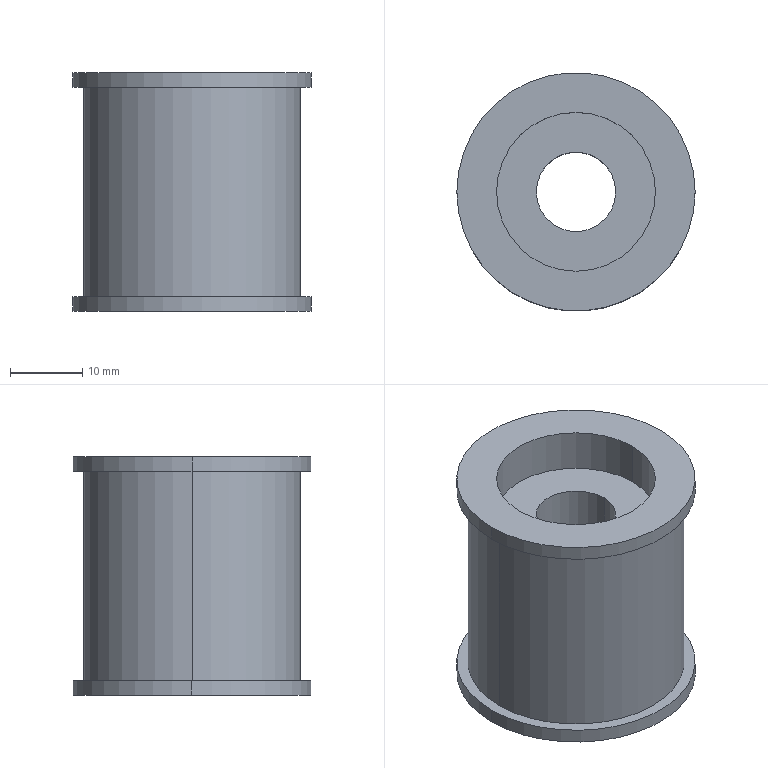Part | STEP file | (PA01.001.LX016) Idler B | 1 solid | 18 faces | box 33 x 33 x 33 mm | volume 17363 mm3 | cylinder 12 | plane 6 | commonest cylinder face diameters 22 x4 33 x4 11 x2 30 x2
STEP:
#1=CARTESIAN_POINT('',(0.,0.,0.));
#2=DIRECTION('',(0.,0.,1.));
#3=DIRECTION('',(1.,0.,0.));
#4=AXIS2_PLACEMENT_3D('',#1,#2,#3);
#5=CARTESIAN_POINT('',(-11.,0.,-10.5));
#6=VERTEX_POINT('',#5);
#7=CARTESIAN_POINT('',(-11.,0.,-16.5));
#8=VERTEX_POINT('',#7);
#9=CARTESIAN_POINT('',(-11.,0.,-10.5));
#10=DIRECTION('',(0.,0.,-1.));
#11=VECTOR('',#10,1.);
#12=LINE('',#9,#11);
#13=CARTESIAN_POINT('',(0.,0.,-10.5));
#14=DIRECTION('',(0.,0.,-1.));
#15=DIRECTION('',(-1.,0.,0.));
#16=AXIS2_PLACEMENT_3D('',#13,#14,#15);
#17=CYLINDRICAL_SURFACE('',#16,11.);
#18=CARTESIAN_POINT('',(6.283,0.));
#19=DIRECTION('',(0.,1.));
#20=VECTOR('',#19,1.);
#21=LINE('',#18,#20);
#22=(GEOMETRIC_REPRESENTATION_CONTEXT(2)PARAMETRIC_REPRESENTATION_CONTEXT()REPRESENTATION_CONTEXT('',''));
#23=DEFINITIONAL_REPRESENTATION('',(#21),#22);
#24=PCURVE('',#17,#23);
#25=CARTESIAN_POINT('',(0.,0.,-10.5));
#26=DIRECTION('',(0.,0.,-1.));
#27=DIRECTION('',(-1.,0.,0.));
#28=AXIS2_PLACEMENT_3D('',#25,#26,#27);
#29=CYLINDRICAL_SURFACE('',#28,11.);
#30=CARTESIAN_POINT('',(0.,0.));
#31=DIRECTION('',(0.,1.));
#32=VECTOR('',#31,1.);
#33=LINE('',#30,#32);
#34=(GEOMETRIC_REPRESENTATION_CONTEXT(2)PARAMETRIC_REPRESENTATION_CONTEXT()REPRESENTATION_CONTEXT('',''));
#35=DEFINITIONAL_REPRESENTATION('',(#33),#34);
#36=PCURVE('',#29,#35);
#37=SURFACE_CURVE('',#12,(#24,#36),.PCURVE_S1.);
#38=EDGE_CURVE('',#6,#8,#37,.T.);
#39=ORIENTED_EDGE('',*,*,#38,.T.);
#40=CARTESIAN_POINT('',(11.,0.,-16.5));
#41=VERTEX_POINT('',#40);
#42=CARTESIAN_POINT('',(0.,0.,-16.5));
#43=DIRECTION('',(0.,0.,-1.));
#44=DIRECTION('',(-1.,0.,0.));
#45=AXIS2_PLACEMENT_3D('',#42,#43,#44);
#46=CIRCLE('',#45,11.);
#47=CARTESIAN_POINT('',(0.,6.));
#48=DIRECTION('',(1.,0.));
#49=VECTOR('',#48,1.);
#50=LINE('',#47,#49);
#51=(GEOMETRIC_REPRESENTATION_CONTEXT(2)PARAMETRIC_REPRESENTATION_CONTEXT()REPRESENTATION_CONTEXT('',''));
#52=DEFINITIONAL_REPRESENTATION('',(#50),#51);
#53=PCURVE('',#17,#52);
#54=CARTESIAN_POINT('',(0.,0.,-16.5));
#55=DIRECTION('',(0.,0.,-1.));
#56=DIRECTION('',(-1.,0.,0.));
#57=AXIS2_PLACEMENT_3D('',#54,#55,#56);
#58=PLANE('',#57);
#59=CARTESIAN_POINT('',(0.,0.));
#60=DIRECTION('',(1.,0.));
#61=AXIS2_PLACEMENT_2D('',#59,#60);
#62=CIRCLE('',#61,11.);
#63=(GEOMETRIC_REPRESENTATION_CONTEXT(2)PARAMETRIC_REPRESENTATION_CONTEXT()REPRESENTATION_CONTEXT('',''));
#64=DEFINITIONAL_REPRESENTATION('',(#62),#63);
#65=PCURVE('',#58,#64);
#66=SURFACE_CURVE('',#46,(#53,#65),.PCURVE_S1.);
#67=EDGE_CURVE('',#41,#8,#66,.T.);
#68=ORIENTED_EDGE('',*,*,#67,.F.);
#69=CARTESIAN_POINT('',(11.,0.,-10.5));
#70=VERTEX_POINT('',#69);
#71=CARTESIAN_POINT('',(11.,0.,-10.5));
#72=DIRECTION('',(0.,0.,-1.));
#73=VECTOR('',#72,1.);
#74=LINE('',#71,#73);
#75=CARTESIAN_POINT('',(3.142,0.));
#76=DIRECTION('',(0.,1.));
#77=VECTOR('',#76,1.);
#78=LINE('',#75,#77);
#79=(GEOMETRIC_REPRESENTATION_CONTEXT(2)PARAMETRIC_REPRESENTATION_CONTEXT()REPRESENTATION_CONTEXT('',''));
#80=DEFINITIONAL_REPRESENTATION('',(#78),#79);
#81=PCURVE('',#17,#80);
#82=CARTESIAN_POINT('',(3.142,0.));
#83=DIRECTION('',(0.,1.));
#84=VECTOR('',#83,1.);
#85=LINE('',#82,#84);
#86=(GEOMETRIC_REPRESENTATION_CONTEXT(2)PARAMETRIC_REPRESENTATION_CONTEXT()REPRESENTATION_CONTEXT('',''));
#87=DEFINITIONAL_REPRESENTATION('',(#85),#86);
#88=PCURVE('',#29,#87);
#89=SURFACE_CURVE('',#74,(#81,#88),.PCURVE_S1.);
#90=EDGE_CURVE('',#70,#41,#89,.T.);
#91=ORIENTED_EDGE('',*,*,#90,.F.);
#92=CARTESIAN_POINT('',(0.,0.,-10.5));
#93=DIRECTION('',(0.,0.,-1.));
#94=DIRECTION('',(-1.,0.,0.));
#95=AXIS2_PLACEMENT_3D('',#92,#93,#94);
#96=CIRCLE('',#95,11.);
#97=CARTESIAN_POINT('',(0.,0.));
#98=DIRECTION('',(1.,0.));
#99=VECTOR('',#98,1.);
#100=LINE('',#97,#99);
#101=(GEOMETRIC_REPRESENTATION_CONTEXT(2)PARAMETRIC_REPRESENTATION_CONTEXT()REPRESENTATION_CONTEXT('',''));
#102=DEFINITIONAL_REPRESENTATION('',(#100),#101);
#103=PCURVE('',#17,#102);
#104=CARTESIAN_POINT('',(0.,0.,-10.5));
#105=DIRECTION('',(0.,0.,-1.));
#106=DIRECTION('',(-1.,0.,0.));
#107=AXIS2_PLACEMENT_3D('',#104,#105,#106);
#108=PLANE('',#107);
#109=CARTESIAN_POINT('',(0.,0.));
#110=DIRECTION('',(1.,0.));
#111=AXIS2_PLACEMENT_2D('',#109,#110);
#112=CIRCLE('',#111,11.);
#113=(GEOMETRIC_REPRESENTATION_CONTEXT(2)PARAMETRIC_REPRESENTATION_CONTEXT()REPRESENTATION_CONTEXT('',''));
#114=DEFINITIONAL_REPRESENTATION('',(#112),#113);
#115=PCURVE('',#108,#114);
#116=SURFACE_CURVE('',#96,(#103,#115),.PCURVE_S1.);
#117=EDGE_CURVE('',#70,#6,#116,.T.);
#118=ORIENTED_EDGE('',*,*,#117,.T.);
#119=EDGE_LOOP('',(#39,#68,#91,#118));
#120=FACE_BOUND('',#119,.F.);
#121=ADVANCED_FACE('',(#120),#17,.F.);
#122=CARTESIAN_POINT('',(11.,0.,10.5));
#123=VERTEX_POINT('',#122);
#124=CARTESIAN_POINT('',(11.,0.,16.5));
#125=VERTEX_POINT('',#124);
#126=CARTESIAN_POINT('',(11.,0.,10.5));
#127=DIRECTION('',(0.,0.,1.));
#128=VECTOR('',#127,1.);
#129=LINE('',#126,#128);
#130=CARTESIAN_POINT('',(0.,0.,10.5));
#131=DIRECTION('',(0.,0.,1.));
#132=DIRECTION('',(1.,0.,0.));
#133=AXIS2_PLACEMENT_3D('',#130,#131,#132);
#134=CYLINDRICAL_SURFACE('',#133,11.);
#135=CARTESIAN_POINT('',(6.283,0.));
#136=DIRECTION('',(0.,1.));
#137=VECTOR('',#136,1.);
#138=LINE('',#135,#137);
#139=(GEOMETRIC_REPRESENTATION_CONTEXT(2)PARAMETRIC_REPRESENTATION_CONTEXT()REPRESENTATION_CONTEXT('',''));
#140=DEFINITIONAL_REPRESENTATION('',(#138),#139);
#141=PCURVE('',#134,#140);
#142=CARTESIAN_POINT('',(0.,0.,10.5));
#143=DIRECTION('',(0.,0.,1.));
#144=DIRECTION('',(1.,0.,0.));
#145=AXIS2_PLACEMENT_3D('',#142,#143,#144);
#146=CYLINDRICAL_SURFACE('',#145,11.);
#147=CARTESIAN_POINT('',(0.,0.));
#148=DIRECTION('',(0.,1.));
#149=VECTOR('',#148,1.);
#150=LINE('',#147,#149);
#151=(GEOMETRIC_REPRESENTATION_CONTEXT(2)PARAMETRIC_REPRESENTATION_CONTEXT()REPRESENTATION_CONTEXT('',''));
#152=DEFINITIONAL_REPRESENTATION('',(#150),#151);
#153=PCURVE('',#146,#152);
#154=SURFACE_CURVE('',#129,(#141,#153),.PCURVE_S1.);
#155=EDGE_CURVE('',#123,#125,#154,.T.);
#156=ORIENTED_EDGE('',*,*,#155,.T.);
#157=CARTESIAN_POINT('',(-11.,0.,16.5));
#158=VERTEX_POINT('',#157);
#159=CARTESIAN_POINT('',(0.,0.,16.5));
#160=DIRECTION('',(0.,0.,1.));
#161=DIRECTION('',(1.,0.,0.));
#162=AXIS2_PLACEMENT_3D('',#159,#160,#161);
#163=CIRCLE('',#162,11.);
#164=CARTESIAN_POINT('',(0.,6.));
#165=DIRECTION('',(1.,0.));
#166=VECTOR('',#165,1.);
#167=LINE('',#164,#166);
#168=(GEOMETRIC_REPRESENTATION_CONTEXT(2)PARAMETRIC_REPRESENTATION_CONTEXT()REPRESENTATION_CONTEXT('',''));
#169=DEFINITIONAL_REPRESENTATION('',(#167),#168);
#170=PCURVE('',#134,#169);
#171=CARTESIAN_POINT('',(0.,0.,16.5));
#172=DIRECTION('',(0.,0.,1.));
#173=DIRECTION('',(1.,0.,0.));
#174=AXIS2_PLACEMENT_3D('',#171,#172,#173);
#175=PLANE('',#174);
#176=CARTESIAN_POINT('',(0.,0.));
#177=DIRECTION('',(1.,0.));
#178=AXIS2_PLACEMENT_2D('',#176,#177);
#179=CIRCLE('',#178,11.);
#180=(GEOMETRIC_REPRESENTATION_CONTEXT(2)PARAMETRIC_REPRESENTATION_CONTEXT()REPRESENTATION_CONTEXT('',''));
#181=DEFINITIONAL_REPRESENTATION('',(#179),#180);
#182=PCURVE('',#175,#181);
#183=SURFACE_CURVE('',#163,(#170,#182),.PCURVE_S1.);
#184=EDGE_CURVE('',#158,#125,#183,.T.);
#185=ORIENTED_EDGE('',*,*,#184,.F.);
#186=CARTESIAN_POINT('',(-11.,0.,10.5));
#187=VERTEX_POINT('',#186);
#188=CARTESIAN_POINT('',(-11.,0.,10.5));
#189=DIRECTION('',(0.,0.,1.));
#190=VECTOR('',#189,1.);
#191=LINE('',#188,#190);
#192=CARTESIAN_POINT('',(3.142,0.));
#193=DIRECTION('',(0.,1.));
#194=VECTOR('',#193,1.);
#195=LINE('',#192,#194);
#196=(GEOMETRIC_REPRESENTATION_CONTEXT(2)PARAMETRIC_REPRESENTATION_CONTEXT()REPRESENTATION_CONTEXT('',''));
#197=DEFINITIONAL_REPRESENTATION('',(#195),#196);
#198=PCURVE('',#134,#197);
#199=CARTESIAN_POINT('',(3.142,0.));
#200=DIRECTION('',(0.,1.));
#201=VECTOR('',#200,1.);
#202=LINE('',#199,#201);
#203=(GEOMETRIC_REPRESENTATION_CONTEXT(2)PARAMETRIC_REPRESENTATION_CONTEXT()REPRESENTATION_CONTEXT('',''));
#204=DEFINITIONAL_REPRESENTATION('',(#202),#203);
#205=PCURVE('',#146,#204);
#206=SURFACE_CURVE('',#191,(#198,#205),.PCURVE_S1.);
#207=EDGE_CURVE('',#187,#158,#206,.T.);
#208=ORIENTED_EDGE('',*,*,#207,.F.);
#209=CARTESIAN_POINT('',(0.,0.,10.5));
#210=DIRECTION('',(0.,0.,1.));
#211=DIRECTION('',(1.,0.,0.));
#212=AXIS2_PLACEMENT_3D('',#209,#210,#211);
#213=CIRCLE('',#212,11.);
#214=CARTESIAN_POINT('',(0.,0.));
#215=DIRECTION('',(1.,0.));
#216=VECTOR('',#215,1.);
#217=LINE('',#214,#216);
#218=(GEOMETRIC_REPRESENTATION_CONTEXT(2)PARAMETRIC_REPRESENTATION_CONTEXT()REPRESENTATION_CONTEXT('',''));
#219=DEFINITIONAL_REPRESENTATION('',(#217),#218);
#220=PCURVE('',#134,#219);
#221=CARTESIAN_POINT('',(0.,0.,10.5));
#222=DIRECTION('',(0.,0.,1.));
#223=DIRECTION('',(1.,0.,0.));
#224=AXIS2_PLACEMENT_3D('',#221,#222,#223);
#225=PLANE('',#224);
#226=CARTESIAN_POINT('',(0.,0.));
#227=DIRECTION('',(1.,0.));
#228=AXIS2_PLACEMENT_2D('',#226,#227);
#229=CIRCLE('',#228,11.);
#230=(GEOMETRIC_REPRESENTATION_CONTEXT(2)PARAMETRIC_REPRESENTATION_CONTEXT()REPRESENTATION_CONTEXT('',''));
#231=DEFINITIONAL_REPRESENTATION('',(#229),#230);
#232=PCURVE('',#225,#231);
#233=SURFACE_CURVE('',#213,(#220,#232),.PCURVE_S1.);
#234=EDGE_CURVE('',#187,#123,#233,.T.);
#235=ORIENTED_EDGE('',*,*,#234,.T.);
#236=EDGE_LOOP('',(#156,#185,#208,#235));
#237=FACE_BOUND('',#236,.F.);
#238=ADVANCED_FACE('',(#237),#134,.F.);
#239=CARTESIAN_POINT('',(-16.5,0.,-16.5));
#240=VERTEX_POINT('',#239);
#241=CARTESIAN_POINT('',(16.5,0.,-16.5));
#242=VERTEX_POINT('',#241);
#243=CARTESIAN_POINT('',(0.,0.,-16.5));
#244=DIRECTION('',(0.,0.,-1.));
#245=DIRECTION('',(-1.,0.,0.));
#246=AXIS2_PLACEMENT_3D('',#243,#244,#245);
#247=CIRCLE('',#246,16.5);
#248=CARTESIAN_POINT('',(0.,0.,-16.5));
#249=DIRECTION('',(0.,0.,1.));
#250=DIRECTION('',(1.,0.,0.));
#251=AXIS2_PLACEMENT_3D('',#248,#249,#250);
#252=CYLINDRICAL_SURFACE('',#251,16.5);
#253=CARTESIAN_POINT('',(3.142,0.));
#254=DIRECTION('',(-1.,0.));
#255=VECTOR('',#254,1.);
#256=LINE('',#253,#255);
#257=(GEOMETRIC_REPRESENTATION_CONTEXT(2)PARAMETRIC_REPRESENTATION_CONTEXT()REPRESENTATION_CONTEXT('',''));
#258=DEFINITIONAL_REPRESENTATION('',(#256),#257);
#259=PCURVE('',#252,#258);
#260=CARTESIAN_POINT('',(0.,0.));
#261=DIRECTION('',(1.,0.));
#262=AXIS2_PLACEMENT_2D('',#260,#261);
#263=CIRCLE('',#262,16.5);
#264=(GEOMETRIC_REPRESENTATION_CONTEXT(2)PARAMETRIC_REPRESENTATION_CONTEXT()REPRESENTATION_CONTEXT('',''));
#265=DEFINITIONAL_REPRESENTATION('',(#263),#264);
#266=PCURVE('',#58,#265);
#267=SURFACE_CURVE('',#247,(#259,#266),.PCURVE_S1.);
#268=EDGE_CURVE('',#240,#242,#267,.T.);
#269=ORIENTED_EDGE('',*,*,#268,.F.);
#270=CARTESIAN_POINT('',(-16.5,0.,-14.5));
#271=VERTEX_POINT('',#270);
#272=CARTESIAN_POINT('',(-16.5,0.,-16.5));
#273=DIRECTION('',(0.,0.,1.));
#274=VECTOR('',#273,1.);
#275=LINE('',#272,#274);
#276=CARTESIAN_POINT('',(3.142,0.));
#277=DIRECTION('',(0.,1.));
#278=VECTOR('',#277,1.);
#279=LINE('',#276,#278);
#280=(GEOMETRIC_REPRESENTATION_CONTEXT(2)PARAMETRIC_REPRESENTATION_CONTEXT()REPRESENTATION_CONTEXT('',''));
#281=DEFINITIONAL_REPRESENTATION('',(#279),#280);
#282=PCURVE('',#252,#281);
#283=CARTESIAN_POINT('',(0.,0.,-16.5));
#284=DIRECTION('',(0.,0.,1.));
#285=DIRECTION('',(1.,0.,0.));
#286=AXIS2_PLACEMENT_3D('',#283,#284,#285);
#287=CYLINDRICAL_SURFACE('',#286,16.5);
#288=CARTESIAN_POINT('',(3.142,0.));
#289=DIRECTION('',(0.,1.));
#290=VECTOR('',#289,1.);
#291=LINE('',#288,#290);
#292=(GEOMETRIC_REPRESENTATION_CONTEXT(2)PARAMETRIC_REPRESENTATION_CONTEXT()REPRESENTATION_CONTEXT('',''));
#293=DEFINITIONAL_REPRESENTATION('',(#291),#292);
#294=PCURVE('',#287,#293);
#295=SURFACE_CURVE('',#275,(#282,#294),.PCURVE_S1.);
#296=EDGE_CURVE('',#240,#271,#295,.T.);
#297=ORIENTED_EDGE('',*,*,#296,.T.);
#298=CARTESIAN_POINT('',(16.5,0.,-14.5));
#299=VERTEX_POINT('',#298);
#300=CARTESIAN_POINT('',(0.,0.,-14.5));
#301=DIRECTION('',(0.,0.,-1.));
#302=DIRECTION('',(-1.,0.,0.));
#303=AXIS2_PLACEMENT_3D('',#300,#301,#302);
#304=CIRCLE('',#303,16.5);
#305=CARTESIAN_POINT('',(3.142,2.));
#306=DIRECTION('',(-1.,0.));
#307=VECTOR('',#306,1.);
#308=LINE('',#305,#307);
#309=(GEOMETRIC_REPRESENTATION_CONTEXT(2)PARAMETRIC_REPRESENTATION_CONTEXT()REPRESENTATION_CONTEXT('',''));
#310=DEFINITIONAL_REPRESENTATION('',(#308),#309);
#311=PCURVE('',#252,#310);
#312=CARTESIAN_POINT('',(0.,0.,-14.5));
#313=DIRECTION('',(0.,0.,-1.));
#314=DIRECTION('',(-1.,0.,0.));
#315=AXIS2_PLACEMENT_3D('',#312,#313,#314);
#316=PLANE('',#315);
#317=CARTESIAN_POINT('',(0.,0.));
#318=DIRECTION('',(1.,0.));
#319=AXIS2_PLACEMENT_2D('',#317,#318);
#320=CIRCLE('',#319,16.5);
#321=(GEOMETRIC_REPRESENTATION_CONTEXT(2)PARAMETRIC_REPRESENTATION_CONTEXT()REPRESENTATION_CONTEXT('',''));
#322=DEFINITIONAL_REPRESENTATION('',(#320),#321);
#323=PCURVE('',#316,#322);
#324=SURFACE_CURVE('',#304,(#311,#323),.PCURVE_S1.);
#325=EDGE_CURVE('',#271,#299,#324,.T.);
#326=ORIENTED_EDGE('',*,*,#325,.T.);
#327=CARTESIAN_POINT('',(16.5,0.,-16.5));
#328=DIRECTION('',(0.,0.,1.));
#329=VECTOR('',#328,1.);
#330=LINE('',#327,#329);
#331=CARTESIAN_POINT('',(0.,0.));
#332=DIRECTION('',(0.,1.));
#333=VECTOR('',#332,1.);
#334=LINE('',#331,#333);
#335=(GEOMETRIC_REPRESENTATION_CONTEXT(2)PARAMETRIC_REPRESENTATION_CONTEXT()REPRESENTATION_CONTEXT('',''));
#336=DEFINITIONAL_REPRESENTATION('',(#334),#335);
#337=PCURVE('',#252,#336);
#338=CARTESIAN_POINT('',(6.283,0.));
#339=DIRECTION('',(0.,1.));
#340=VECTOR('',#339,1.);
#341=LINE('',#338,#340);
#342=(GEOMETRIC_REPRESENTATION_CONTEXT(2)PARAMETRIC_REPRESENTATION_CONTEXT()REPRESENTATION_CONTEXT('',''));
#343=DEFINITIONAL_REPRESENTATION('',(#341),#342);
#344=PCURVE('',#287,#343);
#345=SURFACE_CURVE('',#330,(#337,#344),.PCURVE_S1.);
#346=EDGE_CURVE('',#242,#299,#345,.T.);
#347=ORIENTED_EDGE('',*,*,#346,.F.);
#348=EDGE_LOOP('',(#269,#297,#326,#347));
#349=FACE_BOUND('',#348,.T.);
#350=ADVANCED_FACE('',(#349),#252,.T.);
#351=CARTESIAN_POINT('',(16.5,0.,16.5));
#352=VERTEX_POINT('',#351);
#353=CARTESIAN_POINT('',(-16.5,0.,16.5));
#354=VERTEX_POINT('',#353);
#355=CARTESIAN_POINT('',(0.,0.,16.5));
#356=DIRECTION('',(0.,0.,1.));
#357=DIRECTION('',(1.,0.,0.));
#358=AXIS2_PLACEMENT_3D('',#355,#356,#357);
#359=CIRCLE('',#358,16.5);
#360=CARTESIAN_POINT('',(0.,0.,16.5));
#361=DIRECTION('',(0.,0.,-1.));
#362=DIRECTION('',(-1.,0.,0.));
#363=AXIS2_PLACEMENT_3D('',#360,#361,#362);
#364=CYLINDRICAL_SURFACE('',#363,16.5);
#365=CARTESIAN_POINT('',(3.142,0.));
#366=DIRECTION('',(-1.,0.));
#367=VECTOR('',#366,1.);
#368=LINE('',#365,#367);
#369=(GEOMETRIC_REPRESENTATION_CONTEXT(2)PARAMETRIC_REPRESENTATION_CONTEXT()REPRESENTATION_CONTEXT('',''));
#370=DEFINITIONAL_REPRESENTATION('',(#368),#369);
#371=PCURVE('',#364,#370);
#372=CARTESIAN_POINT('',(0.,0.));
#373=DIRECTION('',(1.,0.));
#374=AXIS2_PLACEMENT_2D('',#372,#373);
#375=CIRCLE('',#374,16.5);
#376=(GEOMETRIC_REPRESENTATION_CONTEXT(2)PARAMETRIC_REPRESENTATION_CONTEXT()REPRESENTATION_CONTEXT('',''));
#377=DEFINITIONAL_REPRESENTATION('',(#375),#376);
#378=PCURVE('',#175,#377);
#379=SURFACE_CURVE('',#359,(#371,#378),.PCURVE_S1.);
#380=EDGE_CURVE('',#352,#354,#379,.T.);
#381=ORIENTED_EDGE('',*,*,#380,.F.);
#382=CARTESIAN_POINT('',(16.5,0.,14.5));
#383=VERTEX_POINT('',#382);
#384=CARTESIAN_POINT('',(16.5,0.,16.5));
#385=DIRECTION('',(0.,0.,-1.));
#386=VECTOR('',#385,1.);
#387=LINE('',#384,#386);
#388=CARTESIAN_POINT('',(3.142,0.));
#389=DIRECTION('',(0.,1.));
#390=VECTOR('',#389,1.);
#391=LINE('',#388,#390);
#392=(GEOMETRIC_REPRESENTATION_CONTEXT(2)PARAMETRIC_REPRESENTATION_CONTEXT()REPRESENTATION_CONTEXT('',''));
#393=DEFINITIONAL_REPRESENTATION('',(#391),#392);
#394=PCURVE('',#364,#393);
#395=CARTESIAN_POINT('',(0.,0.,16.5));
#396=DIRECTION('',(0.,0.,-1.));
#397=DIRECTION('',(-1.,0.,0.));
#398=AXIS2_PLACEMENT_3D('',#395,#396,#397);
#399=CYLINDRICAL_SURFACE('',#398,16.5);
#400=CARTESIAN_POINT('',(3.142,0.));
#401=DIRECTION('',(0.,1.));
#402=VECTOR('',#401,1.);
#403=LINE('',#400,#402);
#404=(GEOMETRIC_REPRESENTATION_CONTEXT(2)PARAMETRIC_REPRESENTATION_CONTEXT()REPRESENTATION_CONTEXT('',''));
#405=DEFINITIONAL_REPRESENTATION('',(#403),#404);
#406=PCURVE('',#399,#405);
#407=SURFACE_CURVE('',#387,(#394,#406),.PCURVE_S1.);
#408=EDGE_CURVE('',#352,#383,#407,.T.);
#409=ORIENTED_EDGE('',*,*,#408,.T.);
#410=CARTESIAN_POINT('',(-16.5,0.,14.5));
#411=VERTEX_POINT('',#410);
#412=CARTESIAN_POINT('',(0.,0.,14.5));
#413=DIRECTION('',(0.,0.,1.));
#414=DIRECTION('',(1.,0.,0.));
#415=AXIS2_PLACEMENT_3D('',#412,#413,#414);
#416=CIRCLE('',#415,16.5);
#417=CARTESIAN_POINT('',(3.142,2.));
#418=DIRECTION('',(-1.,0.));
#419=VECTOR('',#418,1.);
#420=LINE('',#417,#419);
#421=(GEOMETRIC_REPRESENTATION_CONTEXT(2)PARAMETRIC_REPRESENTATION_CONTEXT()REPRESENTATION_CONTEXT('',''));
#422=DEFINITIONAL_REPRESENTATION('',(#420),#421);
#423=PCURVE('',#364,#422);
#424=CARTESIAN_POINT('',(0.,0.,14.5));
#425=DIRECTION('',(0.,0.,1.));
#426=DIRECTION('',(1.,0.,0.));
#427=AXIS2_PLACEMENT_3D('',#424,#425,#426);
#428=PLANE('',#427);
#429=CARTESIAN_POINT('',(0.,0.));
#430=DIRECTION('',(1.,0.));
#431=AXIS2_PLACEMENT_2D('',#429,#430);
#432=CIRCLE('',#431,16.5);
#433=(GEOMETRIC_REPRESENTATION_CONTEXT(2)PARAMETRIC_REPRESENTATION_CONTEXT()REPRESENTATION_CONTEXT('',''));
#434=DEFINITIONAL_REPRESENTATION('',(#432),#433);
#435=PCURVE('',#428,#434);
#436=SURFACE_CURVE('',#416,(#423,#435),.PCURVE_S1.);
#437=EDGE_CURVE('',#383,#411,#436,.T.);
#438=ORIENTED_EDGE('',*,*,#437,.T.);
#439=CARTESIAN_POINT('',(-16.5,0.,16.5));
#440=DIRECTION('',(0.,0.,-1.));
#441=VECTOR('',#440,1.);
#442=LINE('',#439,#441);
#443=CARTESIAN_POINT('',(0.,0.));
#444=DIRECTION('',(0.,1.));
#445=VECTOR('',#444,1.);
#446=LINE('',#443,#445);
#447=(GEOMETRIC_REPRESENTATION_CONTEXT(2)PARAMETRIC_REPRESENTATION_CONTEXT()REPRESENTATION_CONTEXT('',''));
#448=DEFINITIONAL_REPRESENTATION('',(#446),#447);
#449=PCURVE('',#364,#448);
#450=CARTESIAN_POINT('',(6.283,0.));
#451=DIRECTION('',(0.,1.));
#452=VECTOR('',#451,1.);
#453=LINE('',#450,#452);
#454=(GEOMETRIC_REPRESENTATION_CONTEXT(2)PARAMETRIC_REPRESENTATION_CONTEXT()REPRESENTATION_CONTEXT('',''));
#455=DEFINITIONAL_REPRESENTATION('',(#453),#454);
#456=PCURVE('',#399,#455);
#457=SURFACE_CURVE('',#442,(#449,#456),.PCURVE_S1.);
#458=EDGE_CURVE('',#354,#411,#457,.T.);
#459=ORIENTED_EDGE('',*,*,#458,.F.);
#460=EDGE_LOOP('',(#381,#409,#438,#459));
#461=FACE_BOUND('',#460,.T.);
#462=ADVANCED_FACE('',(#461),#364,.T.);
#463=CARTESIAN_POINT('',(15.,0.,14.5));
#464=VERTEX_POINT('',#463);
#465=CARTESIAN_POINT('',(-15.,0.,14.5));
#466=VERTEX_POINT('',#465);
#467=CARTESIAN_POINT('',(0.,0.,14.5));
#468=DIRECTION('',(0.,0.,1.));
#469=DIRECTION('',(1.,0.,0.));
#470=AXIS2_PLACEMENT_3D('',#467,#468,#469);
#471=CIRCLE('',#470,15.);
#472=CARTESIAN_POINT('',(0.,0.,14.5));
#473=DIRECTION('',(0.,0.,-1.));
#474=DIRECTION('',(-1.,0.,0.));
#475=AXIS2_PLACEMENT_3D('',#472,#473,#474);
#476=CYLINDRICAL_SURFACE('',#475,15.);
#477=CARTESIAN_POINT('',(3.142,0.));
#478=DIRECTION('',(-1.,0.));
#479=VECTOR('',#478,1.);
#480=LINE('',#477,#479);
#481=(GEOMETRIC_REPRESENTATION_CONTEXT(2)PARAMETRIC_REPRESENTATION_CONTEXT()REPRESENTATION_CONTEXT('',''));
#482=DEFINITIONAL_REPRESENTATION('',(#480),#481);
#483=PCURVE('',#476,#482);
#484=CARTESIAN_POINT('',(0.,0.));
#485=DIRECTION('',(1.,0.));
#486=AXIS2_PLACEMENT_2D('',#484,#485);
#487=CIRCLE('',#486,15.);
#488=(GEOMETRIC_REPRESENTATION_CONTEXT(2)PARAMETRIC_REPRESENTATION_CONTEXT()REPRESENTATION_CONTEXT('',''));
#489=DEFINITIONAL_REPRESENTATION('',(#487),#488);
#490=PCURVE('',#428,#489);
#491=SURFACE_CURVE('',#471,(#483,#490),.PCURVE_S1.);
#492=EDGE_CURVE('',#464,#466,#491,.T.);
#493=ORIENTED_EDGE('',*,*,#492,.F.);
#494=CARTESIAN_POINT('',(15.,0.,-14.5));
#495=VERTEX_POINT('',#494);
#496=CARTESIAN_POINT('',(15.,0.,14.5));
#497=DIRECTION('',(0.,0.,-1.));
#498=VECTOR('',#497,1.);
#499=LINE('',#496,#498);
#500=CARTESIAN_POINT('',(3.142,0.));
#501=DIRECTION('',(0.,1.));
#502=VECTOR('',#501,1.);
#503=LINE('',#500,#502);
#504=(GEOMETRIC_REPRESENTATION_CONTEXT(2)PARAMETRIC_REPRESENTATION_CONTEXT()REPRESENTATION_CONTEXT('',''));
#505=DEFINITIONAL_REPRESENTATION('',(#503),#504);
#506=PCURVE('',#476,#505);
#507=CARTESIAN_POINT('',(0.,0.,14.5));
#508=DIRECTION('',(0.,0.,-1.));
#509=DIRECTION('',(-1.,0.,0.));
#510=AXIS2_PLACEMENT_3D('',#507,#508,#509);
#511=CYLINDRICAL_SURFACE('',#510,15.);
#512=CARTESIAN_POINT('',(3.142,0.));
#513=DIRECTION('',(0.,1.));
#514=VECTOR('',#513,1.);
#515=LINE('',#512,#514);
#516=(GEOMETRIC_REPRESENTATION_CONTEXT(2)PARAMETRIC_REPRESENTATION_CONTEXT()REPRESENTATION_CONTEXT('',''));
#517=DEFINITIONAL_REPRESENTATION('',(#515),#516);
#518=PCURVE('',#511,#517);
#519=SURFACE_CURVE('',#499,(#506,#518),.PCURVE_S1.);
#520=EDGE_CURVE('',#464,#495,#519,.T.);
#521=ORIENTED_EDGE('',*,*,#520,.T.);
#522=CARTESIAN_POINT('',(-15.,0.,-14.5));
#523=VERTEX_POINT('',#522);
#524=CARTESIAN_POINT('',(0.,0.,-14.5));
#525=DIRECTION('',(0.,0.,-1.));
#526=DIRECTION('',(-1.,0.,0.));
#527=AXIS2_PLACEMENT_3D('',#524,#525,#526);
#528=CIRCLE('',#527,15.);
#529=CARTESIAN_POINT('',(0.,29.));
#530=DIRECTION('',(1.,0.));
#531=VECTOR('',#530,1.);
#532=LINE('',#529,#531);
#533=(GEOMETRIC_REPRESENTATION_CONTEXT(2)PARAMETRIC_REPRESENTATION_CONTEXT()REPRESENTATION_CONTEXT('',''));
#534=DEFINITIONAL_REPRESENTATION('',(#532),#533);
#535=PCURVE('',#476,#534);
#536=CARTESIAN_POINT('',(0.,0.));
#537=DIRECTION('',(1.,0.));
#538=AXIS2_PLACEMENT_2D('',#536,#537);
#539=CIRCLE('',#538,15.);
#540=(GEOMETRIC_REPRESENTATION_CONTEXT(2)PARAMETRIC_REPRESENTATION_CONTEXT()REPRESENTATION_CONTEXT('',''));
#541=DEFINITIONAL_REPRESENTATION('',(#539),#540);
#542=PCURVE('',#316,#541);
#543=SURFACE_CURVE('',#528,(#535,#542),.PCURVE_S1.);
#544=EDGE_CURVE('',#523,#495,#543,.T.);
#545=ORIENTED_EDGE('',*,*,#544,.F.);
#546=CARTESIAN_POINT('',(-15.,0.,14.5));
#547=DIRECTION('',(0.,0.,-1.));
#548=VECTOR('',#547,1.);
#549=LINE('',#546,#548);
#550=CARTESIAN_POINT('',(0.,0.));
#551=DIRECTION('',(0.,1.));
#552=VECTOR('',#551,1.);
#553=LINE('',#550,#552);
#554=(GEOMETRIC_REPRESENTATION_CONTEXT(2)PARAMETRIC_REPRESENTATION_CONTEXT()REPRESENTATION_CONTEXT('',''));
#555=DEFINITIONAL_REPRESENTATION('',(#553),#554);
#556=PCURVE('',#476,#555);
#557=CARTESIAN_POINT('',(6.283,0.));
#558=DIRECTION('',(0.,1.));
#559=VECTOR('',#558,1.);
#560=LINE('',#557,#559);
#561=(GEOMETRIC_REPRESENTATION_CONTEXT(2)PARAMETRIC_REPRESENTATION_CONTEXT()REPRESENTATION_CONTEXT('',''));
#562=DEFINITIONAL_REPRESENTATION('',(#560),#561);
#563=PCURVE('',#511,#562);
#564=SURFACE_CURVE('',#549,(#556,#563),.PCURVE_S1.);
#565=EDGE_CURVE('',#466,#523,#564,.T.);
#566=ORIENTED_EDGE('',*,*,#565,.F.);
#567=EDGE_LOOP('',(#493,#521,#545,#566));
#568=FACE_BOUND('',#567,.T.);
#569=ADVANCED_FACE('',(#568),#476,.T.);
#570=CARTESIAN_POINT('',(5.5,0.,-10.5));
#571=VERTEX_POINT('',#570);
#572=CARTESIAN_POINT('',(5.5,0.,10.5));
#573=VERTEX_POINT('',#572);
#574=CARTESIAN_POINT('',(5.5,0.,-16.5));
#575=DIRECTION('',(0.,0.,1.));
#576=VECTOR('',#575,1.);
#577=LINE('',#574,#576);
#578=CARTESIAN_POINT('',(0.,0.,-16.5));
#579=DIRECTION('',(0.,0.,1.));
#580=DIRECTION('',(1.,0.,0.));
#581=AXIS2_PLACEMENT_3D('',#578,#579,#580);
#582=CYLINDRICAL_SURFACE('',#581,5.5);
#583=CARTESIAN_POINT('',(6.283,0.));
#584=DIRECTION('',(0.,1.));
#585=VECTOR('',#584,1.);
#586=LINE('',#583,#585);
#587=(GEOMETRIC_REPRESENTATION_CONTEXT(2)PARAMETRIC_REPRESENTATION_CONTEXT()REPRESENTATION_CONTEXT('',''));
#588=DEFINITIONAL_REPRESENTATION('',(#586),#587);
#589=PCURVE('',#582,#588);
#590=CARTESIAN_POINT('',(0.,0.,-16.5));
#591=DIRECTION('',(0.,0.,1.));
#592=DIRECTION('',(1.,0.,0.));
#593=AXIS2_PLACEMENT_3D('',#590,#591,#592);
#594=CYLINDRICAL_SURFACE('',#593,5.5);
#595=CARTESIAN_POINT('',(0.,0.));
#596=DIRECTION('',(0.,1.));
#597=VECTOR('',#596,1.);
#598=LINE('',#595,#597);
#599=(GEOMETRIC_REPRESENTATION_CONTEXT(2)PARAMETRIC_REPRESENTATION_CONTEXT()REPRESENTATION_CONTEXT('',''));
#600=DEFINITIONAL_REPRESENTATION('',(#598),#599);
#601=PCURVE('',#594,#600);
#602=SURFACE_CURVE('',#577,(#589,#601),.PCURVE_S1.);
#603=EDGE_CURVE('',#571,#573,#602,.T.);
#604=ORIENTED_EDGE('',*,*,#603,.T.);
#605=CARTESIAN_POINT('',(-5.5,0.,10.5));
#606=VERTEX_POINT('',#605);
#607=CARTESIAN_POINT('',(0.,0.,10.5));
#608=DIRECTION('',(0.,0.,-1.));
#609=DIRECTION('',(1.,0.,0.));
#610=AXIS2_PLACEMENT_3D('',#607,#608,#609);
#611=CIRCLE('',#610,5.5);
#612=CARTESIAN_POINT('',(6.283,27.));
#613=DIRECTION('',(-1.,0.));
#614=VECTOR('',#613,1.);
#615=LINE('',#612,#614);
#616=(GEOMETRIC_REPRESENTATION_CONTEXT(2)PARAMETRIC_REPRESENTATION_CONTEXT()REPRESENTATION_CONTEXT('',''));
#617=DEFINITIONAL_REPRESENTATION('',(#615),#616);
#618=PCURVE('',#582,#617);
#619=CARTESIAN_POINT('',(5.5,0.));
#620=CARTESIAN_POINT('',(5.5,-9.526));
#621=CARTESIAN_POINT('',(-2.75,-4.763));
#622=CARTESIAN_POINT('',(-11.,0.));
#623=CARTESIAN_POINT('',(-2.75,4.763));
#624=CARTESIAN_POINT('',(5.5,9.526));
#625=CARTESIAN_POINT('',(5.5,0.));
#626=(BOUNDED_CURVE()B_SPLINE_CURVE(2,(#619,#620,#621,#622,#623,#624,#625),.UNSPECIFIED.,.T.,.F.)B_SPLINE_CURVE_WITH_KNOTS((1,2,2,2,2,1),(-2.094,0.,2.094,4.189,6.283,8.378),.UNSPECIFIED.)CURVE()GEOMETRIC_REPRESENTATION_ITEM()RATIONAL_B_SPLINE_CURVE((1.,0.5,1.,0.5,1.,0.5,1.))REPRESENTATION_ITEM(''));
#627=(GEOMETRIC_REPRESENTATION_CONTEXT(2)PARAMETRIC_REPRESENTATION_CONTEXT()REPRESENTATION_CONTEXT('',''));
#628=DEFINITIONAL_REPRESENTATION('',(#626),#627);
#629=PCURVE('',#225,#628);
#630=SURFACE_CURVE('',#611,(#618,#629),.PCURVE_S1.);
#631=EDGE_CURVE('',#573,#606,#630,.T.);
#632=ORIENTED_EDGE('',*,*,#631,.T.);
#633=CARTESIAN_POINT('',(-5.5,0.,-10.5));
#634=VERTEX_POINT('',#633);
#635=CARTESIAN_POINT('',(-5.5,0.,-16.5));
#636=DIRECTION('',(0.,0.,1.));
#637=VECTOR('',#636,1.);
#638=LINE('',#635,#637);
#639=CARTESIAN_POINT('',(3.142,0.));
#640=DIRECTION('',(0.,1.));
#641=VECTOR('',#640,1.);
#642=LINE('',#639,#641);
#643=(GEOMETRIC_REPRESENTATION_CONTEXT(2)PARAMETRIC_REPRESENTATION_CONTEXT()REPRESENTATION_CONTEXT('',''));
#644=DEFINITIONAL_REPRESENTATION('',(#642),#643);
#645=PCURVE('',#582,#644);
#646=CARTESIAN_POINT('',(3.142,0.));
#647=DIRECTION('',(0.,1.));
#648=VECTOR('',#647,1.);
#649=LINE('',#646,#648);
#650=(GEOMETRIC_REPRESENTATION_CONTEXT(2)PARAMETRIC_REPRESENTATION_CONTEXT()REPRESENTATION_CONTEXT('',''));
#651=DEFINITIONAL_REPRESENTATION('',(#649),#650);
#652=PCURVE('',#594,#651);
#653=SURFACE_CURVE('',#638,(#645,#652),.PCURVE_S1.);
#654=EDGE_CURVE('',#634,#606,#653,.T.);
#655=ORIENTED_EDGE('',*,*,#654,.F.);
#656=CARTESIAN_POINT('',(0.,0.,-10.5));
#657=DIRECTION('',(0.,0.,1.));
#658=DIRECTION('',(-1.,0.,0.));
#659=AXIS2_PLACEMENT_3D('',#656,#657,#658);
#660=CIRCLE('',#659,5.5);
#661=CARTESIAN_POINT('',(3.142,6.));
#662=DIRECTION('',(1.,0.));
#663=VECTOR('',#662,1.);
#664=LINE('',#661,#663);
#665=(GEOMETRIC_REPRESENTATION_CONTEXT(2)PARAMETRIC_REPRESENTATION_CONTEXT()REPRESENTATION_CONTEXT('',''));
#666=DEFINITIONAL_REPRESENTATION('',(#664),#665);
#667=PCURVE('',#582,#666);
#668=CARTESIAN_POINT('',(5.5,0.));
#669=CARTESIAN_POINT('',(5.5,-9.526));
#670=CARTESIAN_POINT('',(-2.75,-4.763));
#671=CARTESIAN_POINT('',(-11.,0.));
#672=CARTESIAN_POINT('',(-2.75,4.763));
#673=CARTESIAN_POINT('',(5.5,9.526));
#674=CARTESIAN_POINT('',(5.5,0.));
#675=(BOUNDED_CURVE()B_SPLINE_CURVE(2,(#668,#669,#670,#671,#672,#673,#674),.UNSPECIFIED.,.T.,.F.)B_SPLINE_CURVE_WITH_KNOTS((1,2,2,2,2,1),(-2.094,0.,2.094,4.189,6.283,8.378),.UNSPECIFIED.)CURVE()GEOMETRIC_REPRESENTATION_ITEM()RATIONAL_B_SPLINE_CURVE((1.,0.5,1.,0.5,1.,0.5,1.))REPRESENTATION_ITEM(''));
#676=(GEOMETRIC_REPRESENTATION_CONTEXT(2)PARAMETRIC_REPRESENTATION_CONTEXT()REPRESENTATION_CONTEXT('',''));
#677=DEFINITIONAL_REPRESENTATION('',(#675),#676);
#678=PCURVE('',#108,#677);
#679=SURFACE_CURVE('',#660,(#667,#678),.PCURVE_S1.);
#680=EDGE_CURVE('',#634,#571,#679,.T.);
#681=ORIENTED_EDGE('',*,*,#680,.T.);
#682=EDGE_LOOP('',(#604,#632,#655,#681));
#683=FACE_BOUND('',#682,.F.);
#684=ADVANCED_FACE('',(#683),#582,.F.);
#685=CARTESIAN_POINT('',(0.,0.,10.5));
#686=DIRECTION('',(0.,0.,-1.));
#687=DIRECTION('',(1.,0.,0.));
#688=AXIS2_PLACEMENT_3D('',#685,#686,#687);
#689=CIRCLE('',#688,5.5);
#690=CARTESIAN_POINT('',(6.283,27.));
#691=DIRECTION('',(-1.,0.));
#692=VECTOR('',#691,1.);
#693=LINE('',#690,#692);
#694=(GEOMETRIC_REPRESENTATION_CONTEXT(2)PARAMETRIC_REPRESENTATION_CONTEXT()REPRESENTATION_CONTEXT('',''));
#695=DEFINITIONAL_REPRESENTATION('',(#693),#694);
#696=PCURVE('',#594,#695);
#697=CARTESIAN_POINT('',(5.5,0.));
#698=CARTESIAN_POINT('',(5.5,-9.526));
#699=CARTESIAN_POINT('',(-2.75,-4.763));
#700=CARTESIAN_POINT('',(-11.,0.));
#701=CARTESIAN_POINT('',(-2.75,4.763));
#702=CARTESIAN_POINT('',(5.5,9.526));
#703=CARTESIAN_POINT('',(5.5,0.));
#704=(BOUNDED_CURVE()B_SPLINE_CURVE(2,(#697,#698,#699,#700,#701,#702,#703),.UNSPECIFIED.,.T.,.F.)B_SPLINE_CURVE_WITH_KNOTS((1,2,2,2,2,1),(-2.094,0.,2.094,4.189,6.283,8.378),.UNSPECIFIED.)CURVE()GEOMETRIC_REPRESENTATION_ITEM()RATIONAL_B_SPLINE_CURVE((1.,0.5,1.,0.5,1.,0.5,1.))REPRESENTATION_ITEM(''));
#705=(GEOMETRIC_REPRESENTATION_CONTEXT(2)PARAMETRIC_REPRESENTATION_CONTEXT()REPRESENTATION_CONTEXT('',''));
#706=DEFINITIONAL_REPRESENTATION('',(#704),#705);
#707=PCURVE('',#225,#706);
#708=SURFACE_CURVE('',#689,(#696,#707),.PCURVE_S1.);
#709=EDGE_CURVE('',#606,#573,#708,.T.);
#710=ORIENTED_EDGE('',*,*,#709,.T.);
#711=ORIENTED_EDGE('',*,*,#603,.F.);
#712=CARTESIAN_POINT('',(0.,0.,-10.5));
#713=DIRECTION('',(0.,0.,1.));
#714=DIRECTION('',(-1.,0.,0.));
#715=AXIS2_PLACEMENT_3D('',#712,#713,#714);
#716=CIRCLE('',#715,5.5);
#717=CARTESIAN_POINT('',(-3.142,6.));
#718=DIRECTION('',(1.,0.));
#719=VECTOR('',#718,1.);
#720=LINE('',#717,#719);
#721=(GEOMETRIC_REPRESENTATION_CONTEXT(2)PARAMETRIC_REPRESENTATION_CONTEXT()REPRESENTATION_CONTEXT('',''));
#722=DEFINITIONAL_REPRESENTATION('',(#720),#721);
#723=PCURVE('',#594,#722);
#724=CARTESIAN_POINT('',(5.5,0.));
#725=CARTESIAN_POINT('',(5.5,-9.526));
#726=CARTESIAN_POINT('',(-2.75,-4.763));
#727=CARTESIAN_POINT('',(-11.,0.));
#728=CARTESIAN_POINT('',(-2.75,4.763));
#729=CARTESIAN_POINT('',(5.5,9.526));
#730=CARTESIAN_POINT('',(5.5,0.));
#731=(BOUNDED_CURVE()B_SPLINE_CURVE(2,(#724,#725,#726,#727,#728,#729,#730),.UNSPECIFIED.,.T.,.F.)B_SPLINE_CURVE_WITH_KNOTS((1,2,2,2,2,1),(-2.094,0.,2.094,4.189,6.283,8.378),.UNSPECIFIED.)CURVE()GEOMETRIC_REPRESENTATION_ITEM()RATIONAL_B_SPLINE_CURVE((1.,0.5,1.,0.5,1.,0.5,1.))REPRESENTATION_ITEM(''));
#732=(GEOMETRIC_REPRESENTATION_CONTEXT(2)PARAMETRIC_REPRESENTATION_CONTEXT()REPRESENTATION_CONTEXT('',''));
#733=DEFINITIONAL_REPRESENTATION('',(#731),#732);
#734=PCURVE('',#108,#733);
#735=SURFACE_CURVE('',#716,(#723,#734),.PCURVE_S1.);
#736=EDGE_CURVE('',#571,#634,#735,.T.);
#737=ORIENTED_EDGE('',*,*,#736,.T.);
#738=ORIENTED_EDGE('',*,*,#654,.T.);
#739=EDGE_LOOP('',(#710,#711,#737,#738));
#740=FACE_BOUND('',#739,.F.);
#741=ADVANCED_FACE('',(#740),#594,.F.);
#742=ORIENTED_EDGE('',*,*,#520,.F.);
#743=CARTESIAN_POINT('',(0.,0.,14.5));
#744=DIRECTION('',(0.,0.,1.));
#745=DIRECTION('',(1.,0.,0.));
#746=AXIS2_PLACEMENT_3D('',#743,#744,#745);
#747=CIRCLE('',#746,15.);
#748=CARTESIAN_POINT('',(9.425,0.));
#749=DIRECTION('',(-1.,0.));
#750=VECTOR('',#749,1.);
#751=LINE('',#748,#750);
#752=(GEOMETRIC_REPRESENTATION_CONTEXT(2)PARAMETRIC_REPRESENTATION_CONTEXT()REPRESENTATION_CONTEXT('',''));
#753=DEFINITIONAL_REPRESENTATION('',(#751),#752);
#754=PCURVE('',#511,#753);
#755=CARTESIAN_POINT('',(0.,0.));
#756=DIRECTION('',(1.,0.));
#757=AXIS2_PLACEMENT_2D('',#755,#756);
#758=CIRCLE('',#757,15.);
#759=(GEOMETRIC_REPRESENTATION_CONTEXT(2)PARAMETRIC_REPRESENTATION_CONTEXT()REPRESENTATION_CONTEXT('',''));
#760=DEFINITIONAL_REPRESENTATION('',(#758),#759);
#761=PCURVE('',#428,#760);
#762=SURFACE_CURVE('',#747,(#754,#761),.PCURVE_S1.);
#763=EDGE_CURVE('',#466,#464,#762,.T.);
#764=ORIENTED_EDGE('',*,*,#763,.F.);
#765=ORIENTED_EDGE('',*,*,#565,.T.);
#766=CARTESIAN_POINT('',(0.,0.,-14.5));
#767=DIRECTION('',(0.,0.,-1.));
#768=DIRECTION('',(-1.,0.,0.));
#769=AXIS2_PLACEMENT_3D('',#766,#767,#768);
#770=CIRCLE('',#769,15.);
#771=CARTESIAN_POINT('',(0.,29.));
#772=DIRECTION('',(1.,0.));
#773=VECTOR('',#772,1.);
#774=LINE('',#771,#773);
#775=(GEOMETRIC_REPRESENTATION_CONTEXT(2)PARAMETRIC_REPRESENTATION_CONTEXT()REPRESENTATION_CONTEXT('',''));
#776=DEFINITIONAL_REPRESENTATION('',(#774),#775);
#777=PCURVE('',#511,#776);
#778=CARTESIAN_POINT('',(0.,0.));
#779=DIRECTION('',(1.,0.));
#780=AXIS2_PLACEMENT_2D('',#778,#779);
#781=CIRCLE('',#780,15.);
#782=(GEOMETRIC_REPRESENTATION_CONTEXT(2)PARAMETRIC_REPRESENTATION_CONTEXT()REPRESENTATION_CONTEXT('',''));
#783=DEFINITIONAL_REPRESENTATION('',(#781),#782);
#784=PCURVE('',#316,#783);
#785=SURFACE_CURVE('',#770,(#777,#784),.PCURVE_S1.);
#786=EDGE_CURVE('',#495,#523,#785,.T.);
#787=ORIENTED_EDGE('',*,*,#786,.F.);
#788=EDGE_LOOP('',(#742,#764,#765,#787));
#789=FACE_BOUND('',#788,.T.);
#790=ADVANCED_FACE('',(#789),#511,.T.);
#791=CARTESIAN_POINT('',(0.,0.,14.5));
#792=DIRECTION('',(0.,0.,1.));
#793=DIRECTION('',(1.,0.,0.));
#794=AXIS2_PLACEMENT_3D('',#791,#792,#793);
#795=CIRCLE('',#794,16.5);
#796=CARTESIAN_POINT('',(0.,0.));
#797=DIRECTION('',(1.,0.));
#798=AXIS2_PLACEMENT_2D('',#796,#797);
#799=CIRCLE('',#798,16.5);
#800=(GEOMETRIC_REPRESENTATION_CONTEXT(2)PARAMETRIC_REPRESENTATION_CONTEXT()REPRESENTATION_CONTEXT('',''));
#801=DEFINITIONAL_REPRESENTATION('',(#799),#800);
#802=PCURVE('',#428,#801);
#803=CARTESIAN_POINT('',(9.425,2.));
#804=DIRECTION('',(-1.,0.));
#805=VECTOR('',#804,1.);
#806=LINE('',#803,#805);
#807=(GEOMETRIC_REPRESENTATION_CONTEXT(2)PARAMETRIC_REPRESENTATION_CONTEXT()REPRESENTATION_CONTEXT('',''));
#808=DEFINITIONAL_REPRESENTATION('',(#806),#807);
#809=PCURVE('',#399,#808);
#810=SURFACE_CURVE('',#795,(#802,#809),.PCURVE_S1.);
#811=EDGE_CURVE('',#411,#383,#810,.T.);
#812=ORIENTED_EDGE('',*,*,#811,.F.);
#813=ORIENTED_EDGE('',*,*,#437,.F.);
#814=EDGE_LOOP('',(#812,#813));
#815=FACE_BOUND('',#814,.T.);
#816=ORIENTED_EDGE('',*,*,#763,.T.);
#817=ORIENTED_EDGE('',*,*,#492,.T.);
#818=EDGE_LOOP('',(#816,#817));
#819=FACE_BOUND('',#818,.T.);
#820=ADVANCED_FACE('',(#815,#819),#428,.F.);
#821=ORIENTED_EDGE('',*,*,#408,.F.);
#822=CARTESIAN_POINT('',(0.,0.,16.5));
#823=DIRECTION('',(0.,0.,1.));
#824=DIRECTION('',(1.,0.,0.));
#825=AXIS2_PLACEMENT_3D('',#822,#823,#824);
#826=CIRCLE('',#825,16.5);
#827=CARTESIAN_POINT('',(9.425,0.));
#828=DIRECTION('',(-1.,0.));
#829=VECTOR('',#828,1.);
#830=LINE('',#827,#829);
#831=(GEOMETRIC_REPRESENTATION_CONTEXT(2)PARAMETRIC_REPRESENTATION_CONTEXT()REPRESENTATION_CONTEXT('',''));
#832=DEFINITIONAL_REPRESENTATION('',(#830),#831);
#833=PCURVE('',#399,#832);
#834=CARTESIAN_POINT('',(0.,0.));
#835=DIRECTION('',(1.,0.));
#836=AXIS2_PLACEMENT_2D('',#834,#835);
#837=CIRCLE('',#836,16.5);
#838=(GEOMETRIC_REPRESENTATION_CONTEXT(2)PARAMETRIC_REPRESENTATION_CONTEXT()REPRESENTATION_CONTEXT('',''));
#839=DEFINITIONAL_REPRESENTATION('',(#837),#838);
#840=PCURVE('',#175,#839);
#841=SURFACE_CURVE('',#826,(#833,#840),.PCURVE_S1.);
#842=EDGE_CURVE('',#354,#352,#841,.T.);
#843=ORIENTED_EDGE('',*,*,#842,.F.);
#844=ORIENTED_EDGE('',*,*,#458,.T.);
#845=ORIENTED_EDGE('',*,*,#811,.T.);
#846=EDGE_LOOP('',(#821,#843,#844,#845));
#847=FACE_BOUND('',#846,.T.);
#848=ADVANCED_FACE('',(#847),#399,.T.);
#849=CARTESIAN_POINT('',(0.,0.,16.5));
#850=DIRECTION('',(0.,0.,1.));
#851=DIRECTION('',(1.,0.,0.));
#852=AXIS2_PLACEMENT_3D('',#849,#850,#851);
#853=CIRCLE('',#852,11.);
#854=CARTESIAN_POINT('',(0.,0.));
#855=DIRECTION('',(1.,0.));
#856=AXIS2_PLACEMENT_2D('',#854,#855);
#857=CIRCLE('',#856,11.);
#858=(GEOMETRIC_REPRESENTATION_CONTEXT(2)PARAMETRIC_REPRESENTATION_CONTEXT()REPRESENTATION_CONTEXT('',''));
#859=DEFINITIONAL_REPRESENTATION('',(#857),#858);
#860=PCURVE('',#175,#859);
#861=CARTESIAN_POINT('',(0.,6.));
#862=DIRECTION('',(1.,0.));
#863=VECTOR('',#862,1.);
#864=LINE('',#861,#863);
#865=(GEOMETRIC_REPRESENTATION_CONTEXT(2)PARAMETRIC_REPRESENTATION_CONTEXT()REPRESENTATION_CONTEXT('',''));
#866=DEFINITIONAL_REPRESENTATION('',(#864),#865);
#867=PCURVE('',#146,#866);
#868=SURFACE_CURVE('',#853,(#860,#867),.PCURVE_S1.);
#869=EDGE_CURVE('',#125,#158,#868,.T.);
#870=ORIENTED_EDGE('',*,*,#869,.F.);
#871=ORIENTED_EDGE('',*,*,#184,.F.);
#872=EDGE_LOOP('',(#870,#871));
#873=FACE_BOUND('',#872,.T.);
#874=ORIENTED_EDGE('',*,*,#842,.T.);
#875=ORIENTED_EDGE('',*,*,#380,.T.);
#876=EDGE_LOOP('',(#874,#875));
#877=FACE_BOUND('',#876,.T.);
#878=ADVANCED_FACE('',(#873,#877),#175,.T.);
#879=CARTESIAN_POINT('',(0.,0.,-14.5));
#880=DIRECTION('',(0.,0.,-1.));
#881=DIRECTION('',(-1.,0.,0.));
#882=AXIS2_PLACEMENT_3D('',#879,#880,#881);
#883=CIRCLE('',#882,16.5);
#884=CARTESIAN_POINT('',(0.,0.));
#885=DIRECTION('',(1.,0.));
#886=AXIS2_PLACEMENT_2D('',#884,#885);
#887=CIRCLE('',#886,16.5);
#888=(GEOMETRIC_REPRESENTATION_CONTEXT(2)PARAMETRIC_REPRESENTATION_CONTEXT()REPRESENTATION_CONTEXT('',''));
#889=DEFINITIONAL_REPRESENTATION('',(#887),#888);
#890=PCURVE('',#316,#889);
#891=CARTESIAN_POINT('',(9.425,2.));
#892=DIRECTION('',(-1.,0.));
#893=VECTOR('',#892,1.);
#894=LINE('',#891,#893);
#895=(GEOMETRIC_REPRESENTATION_CONTEXT(2)PARAMETRIC_REPRESENTATION_CONTEXT()REPRESENTATION_CONTEXT('',''));
#896=DEFINITIONAL_REPRESENTATION('',(#894),#895);
#897=PCURVE('',#287,#896);
#898=SURFACE_CURVE('',#883,(#890,#897),.PCURVE_S1.);
#899=EDGE_CURVE('',#299,#271,#898,.T.);
#900=ORIENTED_EDGE('',*,*,#899,.F.);
#901=ORIENTED_EDGE('',*,*,#325,.F.);
#902=EDGE_LOOP('',(#900,#901));
#903=FACE_BOUND('',#902,.T.);
#904=ORIENTED_EDGE('',*,*,#544,.T.);
#905=ORIENTED_EDGE('',*,*,#786,.T.);
#906=EDGE_LOOP('',(#904,#905));
#907=FACE_BOUND('',#906,.T.);
#908=ADVANCED_FACE('',(#903,#907),#316,.F.);
#909=ORIENTED_EDGE('',*,*,#296,.F.);
#910=CARTESIAN_POINT('',(0.,0.,-16.5));
#911=DIRECTION('',(0.,0.,-1.));
#912=DIRECTION('',(-1.,0.,0.));
#913=AXIS2_PLACEMENT_3D('',#910,#911,#912);
#914=CIRCLE('',#913,16.5);
#915=CARTESIAN_POINT('',(9.425,0.));
#916=DIRECTION('',(-1.,0.));
#917=VECTOR('',#916,1.);
#918=LINE('',#915,#917);
#919=(GEOMETRIC_REPRESENTATION_CONTEXT(2)PARAMETRIC_REPRESENTATION_CONTEXT()REPRESENTATION_CONTEXT('',''));
#920=DEFINITIONAL_REPRESENTATION('',(#918),#919);
#921=PCURVE('',#287,#920);
#922=CARTESIAN_POINT('',(0.,0.));
#923=DIRECTION('',(1.,0.));
#924=AXIS2_PLACEMENT_2D('',#922,#923);
#925=CIRCLE('',#924,16.5);
#926=(GEOMETRIC_REPRESENTATION_CONTEXT(2)PARAMETRIC_REPRESENTATION_CONTEXT()REPRESENTATION_CONTEXT('',''));
#927=DEFINITIONAL_REPRESENTATION('',(#925),#926);
#928=PCURVE('',#58,#927);
#929=SURFACE_CURVE('',#914,(#921,#928),.PCURVE_S1.);
#930=EDGE_CURVE('',#242,#240,#929,.T.);
#931=ORIENTED_EDGE('',*,*,#930,.F.);
#932=ORIENTED_EDGE('',*,*,#346,.T.);
#933=ORIENTED_EDGE('',*,*,#899,.T.);
#934=EDGE_LOOP('',(#909,#931,#932,#933));
#935=FACE_BOUND('',#934,.T.);
#936=ADVANCED_FACE('',(#935),#287,.T.);
#937=CARTESIAN_POINT('',(0.,0.,-16.5));
#938=DIRECTION('',(0.,0.,-1.));
#939=DIRECTION('',(-1.,0.,0.));
#940=AXIS2_PLACEMENT_3D('',#937,#938,#939);
#941=CIRCLE('',#940,11.);
#942=CARTESIAN_POINT('',(0.,0.));
#943=DIRECTION('',(1.,0.));
#944=AXIS2_PLACEMENT_2D('',#942,#943);
#945=CIRCLE('',#944,11.);
#946=(GEOMETRIC_REPRESENTATION_CONTEXT(2)PARAMETRIC_REPRESENTATION_CONTEXT()REPRESENTATION_CONTEXT('',''));
#947=DEFINITIONAL_REPRESENTATION('',(#945),#946);
#948=PCURVE('',#58,#947);
#949=CARTESIAN_POINT('',(0.,6.));
#950=DIRECTION('',(1.,0.));
#951=VECTOR('',#950,1.);
#952=LINE('',#949,#951);
#953=(GEOMETRIC_REPRESENTATION_CONTEXT(2)PARAMETRIC_REPRESENTATION_CONTEXT()REPRESENTATION_CONTEXT('',''));
#954=DEFINITIONAL_REPRESENTATION('',(#952),#953);
#955=PCURVE('',#29,#954);
#956=SURFACE_CURVE('',#941,(#948,#955),.PCURVE_S1.);
#957=EDGE_CURVE('',#8,#41,#956,.T.);
#958=ORIENTED_EDGE('',*,*,#957,.F.);
#959=ORIENTED_EDGE('',*,*,#67,.F.);
#960=EDGE_LOOP('',(#958,#959));
#961=FACE_BOUND('',#960,.T.);
#962=ORIENTED_EDGE('',*,*,#930,.T.);
#963=ORIENTED_EDGE('',*,*,#268,.T.);
#964=EDGE_LOOP('',(#962,#963));
#965=FACE_BOUND('',#964,.T.);
#966=ADVANCED_FACE('',(#961,#965),#58,.T.);
#967=CARTESIAN_POINT('',(0.,0.,10.5));
#968=DIRECTION('',(0.,0.,1.));
#969=DIRECTION('',(1.,0.,0.));
#970=AXIS2_PLACEMENT_3D('',#967,#968,#969);
#971=CIRCLE('',#970,11.);
#972=CARTESIAN_POINT('',(0.,0.));
#973=DIRECTION('',(1.,0.));
#974=AXIS2_PLACEMENT_2D('',#972,#973);
#975=CIRCLE('',#974,11.);
#976=(GEOMETRIC_REPRESENTATION_CONTEXT(2)PARAMETRIC_REPRESENTATION_CONTEXT()REPRESENTATION_CONTEXT('',''));
#977=DEFINITIONAL_REPRESENTATION('',(#975),#976);
#978=PCURVE('',#225,#977);
#979=CARTESIAN_POINT('',(0.,0.));
#980=DIRECTION('',(1.,0.));
#981=VECTOR('',#980,1.);
#982=LINE('',#979,#981);
#983=(GEOMETRIC_REPRESENTATION_CONTEXT(2)PARAMETRIC_REPRESENTATION_CONTEXT()REPRESENTATION_CONTEXT('',''));
#984=DEFINITIONAL_REPRESENTATION('',(#982),#983);
#985=PCURVE('',#146,#984);
#986=SURFACE_CURVE('',#971,(#978,#985),.PCURVE_S1.);
#987=EDGE_CURVE('',#123,#187,#986,.T.);
#988=ORIENTED_EDGE('',*,*,#987,.T.);
#989=ORIENTED_EDGE('',*,*,#234,.T.);
#990=EDGE_LOOP('',(#988,#989));
#991=FACE_BOUND('',#990,.T.);
#992=ORIENTED_EDGE('',*,*,#631,.T.);
#993=ORIENTED_EDGE('',*,*,#709,.T.);
#994=EDGE_LOOP('',(#992,#993));
#995=FACE_BOUND('',#994,.T.);
#996=ADVANCED_FACE('',(#991,#995),#225,.T.);
#997=ORIENTED_EDGE('',*,*,#869,.F.);
#998=ORIENTED_EDGE('',*,*,#155,.F.);
#999=ORIENTED_EDGE('',*,*,#987,.T.);
#1000=ORIENTED_EDGE('',*,*,#207,.T.);
#1001=EDGE_LOOP('',(#997,#998,#999,#1000));
#1002=FACE_BOUND('',#1001,.F.);
#1003=ADVANCED_FACE('',(#1002),#146,.F.);
#1004=CARTESIAN_POINT('',(0.,0.,-10.5));
#1005=DIRECTION('',(0.,0.,-1.));
#1006=DIRECTION('',(-1.,0.,0.));
#1007=AXIS2_PLACEMENT_3D('',#1004,#1005,#1006);
#1008=CIRCLE('',#1007,11.);
#1009=CARTESIAN_POINT('',(0.,0.));
#1010=DIRECTION('',(1.,0.));
#1011=AXIS2_PLACEMENT_2D('',#1009,#1010);
#1012=CIRCLE('',#1011,11.);
#1013=(GEOMETRIC_REPRESENTATION_CONTEXT(2)PARAMETRIC_REPRESENTATION_CONTEXT()REPRESENTATION_CONTEXT('',''));
#1014=DEFINITIONAL_REPRESENTATION('',(#1012),#1013);
#1015=PCURVE('',#108,#1014);
#1016=CARTESIAN_POINT('',(0.,0.));
#1017=DIRECTION('',(1.,0.));
#1018=VECTOR('',#1017,1.);
#1019=LINE('',#1016,#1018);
#1020=(GEOMETRIC_REPRESENTATION_CONTEXT(2)PARAMETRIC_REPRESENTATION_CONTEXT()REPRESENTATION_CONTEXT('',''));
#1021=DEFINITIONAL_REPRESENTATION('',(#1019),#1020);
#1022=PCURVE('',#29,#1021);
#1023=SURFACE_CURVE('',#1008,(#1015,#1022),.PCURVE_S1.);
#1024=EDGE_CURVE('',#6,#70,#1023,.T.);
#1025=ORIENTED_EDGE('',*,*,#1024,.T.);
#1026=ORIENTED_EDGE('',*,*,#117,.T.);
#1027=EDGE_LOOP('',(#1025,#1026));
#1028=FACE_BOUND('',#1027,.T.);
#1029=ORIENTED_EDGE('',*,*,#736,.T.);
#1030=ORIENTED_EDGE('',*,*,#680,.T.);
#1031=EDGE_LOOP('',(#1029,#1030));
#1032=FACE_BOUND('',#1031,.T.);
#1033=ADVANCED_FACE('',(#1028,#1032),#108,.T.);
#1034=ORIENTED_EDGE('',*,*,#957,.F.);
#1035=ORIENTED_EDGE('',*,*,#38,.F.);
#1036=ORIENTED_EDGE('',*,*,#1024,.T.);
#1037=ORIENTED_EDGE('',*,*,#90,.T.);
#1038=EDGE_LOOP('',(#1034,#1035,#1036,#1037));
#1039=FACE_BOUND('',#1038,.F.);
#1040=ADVANCED_FACE('',(#1039),#29,.F.);
#1041=CLOSED_SHELL('',(#121,#238,#350,#462,#569,#684,#741,#790,#820,#848,#878,#908,#936,#966,#996,#1003,#1033,#1040));
#1042=MANIFOLD_SOLID_BREP('',#1041);
#1043=(LENGTH_UNIT()NAMED_UNIT(*)SI_UNIT(.MILLI.,.METRE.));
#1044=UNCERTAINTY_MEASURE_WITH_UNIT(LENGTH_MEASURE(0.0000001),#1043,'','');
#1045=(NAMED_UNIT(*)PLANE_ANGLE_UNIT()SI_UNIT($,.RADIAN.));
#1046=(NAMED_UNIT(*)SI_UNIT($,.STERADIAN.)SOLID_ANGLE_UNIT());
#1047=(GEOMETRIC_REPRESENTATION_CONTEXT(3)GLOBAL_UNCERTAINTY_ASSIGNED_CONTEXT((#1044))GLOBAL_UNIT_ASSIGNED_CONTEXT((#1043,#1045,#1046))REPRESENTATION_CONTEXT('',''));
#1048=ADVANCED_BREP_SHAPE_REPRESENTATION('',(#4,#1042),#1047);